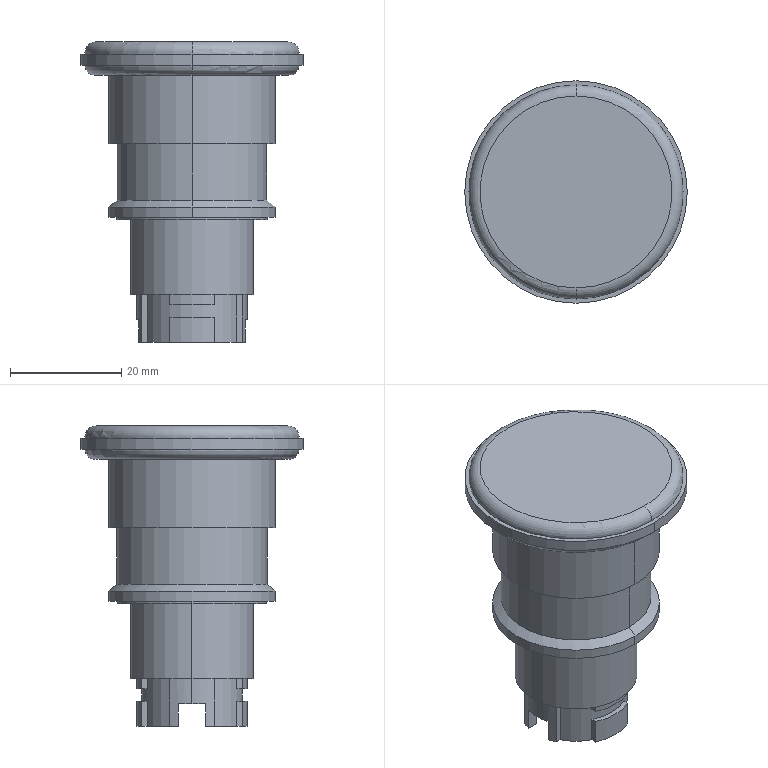Part | STEP file | A22NE_M_N_BASE | 1 solid | 64 faces | box 40 x 40 x 54 mm | volume 28199 mm3 | plane 32 | cylinder 26 | torus 4 | cone 2 | commonest cylinder face diameters 19.8 x8 27 x4 30 x4 12.6 x2 15.7 x2 18 x2